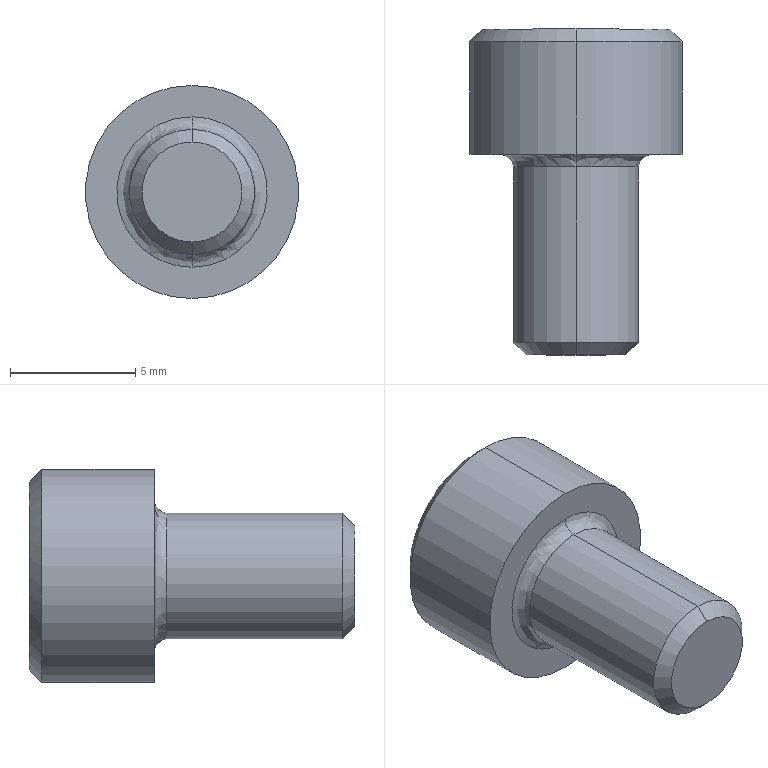Part | STEP file | 1 solid | 20 faces | box 8.5 x 13 x 8.5 mm | volume 400.62 mm3 | plane 10 | cone 4 | cylinder 4 | spline 2 | commonest cylinder face diameters 5 x2 8.5 x2
STEP:
#1=CARTESIAN_POINT('',(0.,0.,0.));
#2=DIRECTION('',(0.,0.,1.));
#3=DIRECTION('',(1.,0.,0.));
#4=AXIS2_PLACEMENT_3D('',#1,#2,#3);
#5=CARTESIAN_POINT('',(0.,-8.,2.));
#6=VERTEX_POINT('',#5);
#7=CARTESIAN_POINT('',(0.,-8.,-2.));
#8=VERTEX_POINT('',#7);
#9=CARTESIAN_POINT('',(0.,-8.,0.));
#10=DIRECTION('',(0.,1.,0.));
#11=DIRECTION('',(0.,0.,1.));
#12=AXIS2_PLACEMENT_3D('',#9,#10,#11);
#13=CIRCLE('',#12,2.);
#14=CARTESIAN_POINT('',(0.,-8.,0.));
#15=DIRECTION('',(0.,-1.,0.));
#16=DIRECTION('',(0.,0.,-1.));
#17=AXIS2_PLACEMENT_3D('',#14,#15,#16);
#18=PLANE('',#17);
#19=CARTESIAN_POINT('',(-2.,0.));
#20=CARTESIAN_POINT('',(-2.,3.464));
#21=CARTESIAN_POINT('',(1.,1.732));
#22=CARTESIAN_POINT('',(4.,0.));
#23=CARTESIAN_POINT('',(1.,-1.732));
#24=CARTESIAN_POINT('',(-2.,-3.464));
#25=CARTESIAN_POINT('',(-2.,0.));
#26=(BOUNDED_CURVE()B_SPLINE_CURVE(2,(#19,#20,#21,#22,#23,#24,#25),.UNSPECIFIED.,.T.,.F.)B_SPLINE_CURVE_WITH_KNOTS((1,2,2,2,2,1),(-2.094,0.,2.094,4.189,6.283,8.378),.UNSPECIFIED.)CURVE()GEOMETRIC_REPRESENTATION_ITEM()RATIONAL_B_SPLINE_CURVE((1.,0.5,1.,0.5,1.,0.5,1.))REPRESENTATION_ITEM(''));
#27=(GEOMETRIC_REPRESENTATION_CONTEXT(2)PARAMETRIC_REPRESENTATION_CONTEXT()REPRESENTATION_CONTEXT('',''));
#28=DEFINITIONAL_REPRESENTATION('',(#26),#27);
#29=PCURVE('',#18,#28);
#30=CARTESIAN_POINT('',(0.,-7.5,0.));
#31=DIRECTION('',(0.,1.,0.));
#32=DIRECTION('',(0.,0.,1.));
#33=AXIS2_PLACEMENT_3D('',#30,#31,#32);
#34=CONICAL_SURFACE('',#33,2.5,0.7854);
#35=CARTESIAN_POINT('',(0.,-0.5));
#36=DIRECTION('',(1.,0.));
#37=VECTOR('',#36,1.);
#38=LINE('',#35,#37);
#39=(GEOMETRIC_REPRESENTATION_CONTEXT(2)PARAMETRIC_REPRESENTATION_CONTEXT()REPRESENTATION_CONTEXT('',''));
#40=DEFINITIONAL_REPRESENTATION('',(#38),#39);
#41=PCURVE('',#34,#40);
#42=SURFACE_CURVE('',#13,(#29,#41),.PCURVE_S1.);
#43=EDGE_CURVE('',#6,#8,#42,.T.);
#44=ORIENTED_EDGE('',*,*,#43,.F.);
#45=CARTESIAN_POINT('',(0.,-8.,0.));
#46=DIRECTION('',(0.,1.,0.));
#47=DIRECTION('',(0.,0.,1.));
#48=AXIS2_PLACEMENT_3D('',#45,#46,#47);
#49=CIRCLE('',#48,2.);
#50=CARTESIAN_POINT('',(-2.,0.));
#51=CARTESIAN_POINT('',(-2.,3.464));
#52=CARTESIAN_POINT('',(1.,1.732));
#53=CARTESIAN_POINT('',(4.,0.));
#54=CARTESIAN_POINT('',(1.,-1.732));
#55=CARTESIAN_POINT('',(-2.,-3.464));
#56=CARTESIAN_POINT('',(-2.,0.));
#57=(BOUNDED_CURVE()B_SPLINE_CURVE(2,(#50,#51,#52,#53,#54,#55,#56),.UNSPECIFIED.,.T.,.F.)B_SPLINE_CURVE_WITH_KNOTS((1,2,2,2,2,1),(-2.094,0.,2.094,4.189,6.283,8.378),.UNSPECIFIED.)CURVE()GEOMETRIC_REPRESENTATION_ITEM()RATIONAL_B_SPLINE_CURVE((1.,0.5,1.,0.5,1.,0.5,1.))REPRESENTATION_ITEM(''));
#58=(GEOMETRIC_REPRESENTATION_CONTEXT(2)PARAMETRIC_REPRESENTATION_CONTEXT()REPRESENTATION_CONTEXT('',''));
#59=DEFINITIONAL_REPRESENTATION('',(#57),#58);
#60=PCURVE('',#18,#59);
#61=CARTESIAN_POINT('',(0.,-7.5,0.));
#62=DIRECTION('',(0.,1.,0.));
#63=DIRECTION('',(0.,0.,1.));
#64=AXIS2_PLACEMENT_3D('',#61,#62,#63);
#65=CONICAL_SURFACE('',#64,2.5,0.7854);
#66=CARTESIAN_POINT('',(0.,-0.5));
#67=DIRECTION('',(1.,0.));
#68=VECTOR('',#67,1.);
#69=LINE('',#66,#68);
#70=(GEOMETRIC_REPRESENTATION_CONTEXT(2)PARAMETRIC_REPRESENTATION_CONTEXT()REPRESENTATION_CONTEXT('',''));
#71=DEFINITIONAL_REPRESENTATION('',(#69),#70);
#72=PCURVE('',#65,#71);
#73=SURFACE_CURVE('',#49,(#60,#72),.PCURVE_S1.);
#74=EDGE_CURVE('',#8,#6,#73,.T.);
#75=ORIENTED_EDGE('',*,*,#74,.F.);
#76=EDGE_LOOP('',(#44,#75));
#77=FACE_BOUND('',#76,.T.);
#78=ADVANCED_FACE('',(#77),#18,.T.);
#79=CARTESIAN_POINT('',(-1.155,2.4,2.));
#80=VERTEX_POINT('',#79);
#81=CARTESIAN_POINT('',(1.155,2.4,2.));
#82=VERTEX_POINT('',#81);
#83=CARTESIAN_POINT('',(-1.155,2.4,2.));
#84=DIRECTION('',(1.,0.,0.));
#85=VECTOR('',#84,1.);
#86=LINE('',#83,#85);
#87=CARTESIAN_POINT('',(0.,2.4,0.));
#88=DIRECTION('',(0.,1.,0.));
#89=DIRECTION('',(1.,0.,0.));
#90=AXIS2_PLACEMENT_3D('',#87,#88,#89);
#91=PLANE('',#90);
#92=CARTESIAN_POINT('',(-1.155,-2.));
#93=DIRECTION('',(1.,0.));
#94=VECTOR('',#93,1.);
#95=LINE('',#92,#94);
#96=(GEOMETRIC_REPRESENTATION_CONTEXT(2)PARAMETRIC_REPRESENTATION_CONTEXT()REPRESENTATION_CONTEXT('',''));
#97=DEFINITIONAL_REPRESENTATION('',(#95),#96);
#98=PCURVE('',#91,#97);
#99=CARTESIAN_POINT('',(-1.155,2.4,2.));
#100=DIRECTION('',(0.,0.,1.));
#101=DIRECTION('',(1.,0.,0.));
#102=AXIS2_PLACEMENT_3D('',#99,#100,#101);
#103=PLANE('',#102);
#104=CARTESIAN_POINT('',(0.,0.));
#105=DIRECTION('',(1.,0.));
#106=VECTOR('',#105,1.);
#107=LINE('',#104,#106);
#108=(GEOMETRIC_REPRESENTATION_CONTEXT(2)PARAMETRIC_REPRESENTATION_CONTEXT()REPRESENTATION_CONTEXT('',''));
#109=DEFINITIONAL_REPRESENTATION('',(#107),#108);
#110=PCURVE('',#103,#109);
#111=SURFACE_CURVE('',#86,(#98,#110),.PCURVE_S1.);
#112=EDGE_CURVE('',#80,#82,#111,.T.);
#113=ORIENTED_EDGE('',*,*,#112,.T.);
#114=CARTESIAN_POINT('',(2.309,2.4,0.));
#115=VERTEX_POINT('',#114);
#116=CARTESIAN_POINT('',(1.155,2.4,2.));
#117=DIRECTION('',(0.5,0.,-0.866));
#118=VECTOR('',#117,1.);
#119=LINE('',#116,#118);
#120=CARTESIAN_POINT('',(1.155,-2.));
#121=DIRECTION('',(0.5,0.866));
#122=VECTOR('',#121,1.);
#123=LINE('',#120,#122);
#124=(GEOMETRIC_REPRESENTATION_CONTEXT(2)PARAMETRIC_REPRESENTATION_CONTEXT()REPRESENTATION_CONTEXT('',''));
#125=DEFINITIONAL_REPRESENTATION('',(#123),#124);
#126=PCURVE('',#91,#125);
#127=CARTESIAN_POINT('',(1.155,2.4,2.));
#128=DIRECTION('',(0.866,0.,0.5));
#129=DIRECTION('',(0.,-1.,0.));
#130=AXIS2_PLACEMENT_3D('',#127,#128,#129);
#131=PLANE('',#130);
#132=CARTESIAN_POINT('',(0.,0.));
#133=DIRECTION('',(0.,1.));
#134=VECTOR('',#133,1.);
#135=LINE('',#132,#134);
#136=(GEOMETRIC_REPRESENTATION_CONTEXT(2)PARAMETRIC_REPRESENTATION_CONTEXT()REPRESENTATION_CONTEXT('',''));
#137=DEFINITIONAL_REPRESENTATION('',(#135),#136);
#138=PCURVE('',#131,#137);
#139=SURFACE_CURVE('',#119,(#126,#138),.PCURVE_S1.);
#140=EDGE_CURVE('',#82,#115,#139,.T.);
#141=ORIENTED_EDGE('',*,*,#140,.T.);
#142=CARTESIAN_POINT('',(1.155,2.4,-2.));
#143=VERTEX_POINT('',#142);
#144=CARTESIAN_POINT('',(2.309,2.4,0.));
#145=DIRECTION('',(-0.5,0.,-0.866));
#146=VECTOR('',#145,1.);
#147=LINE('',#144,#146);
#148=CARTESIAN_POINT('',(2.309,0.));
#149=DIRECTION('',(-0.5,0.866));
#150=VECTOR('',#149,1.);
#151=LINE('',#148,#150);
#152=(GEOMETRIC_REPRESENTATION_CONTEXT(2)PARAMETRIC_REPRESENTATION_CONTEXT()REPRESENTATION_CONTEXT('',''));
#153=DEFINITIONAL_REPRESENTATION('',(#151),#152);
#154=PCURVE('',#91,#153);
#155=CARTESIAN_POINT('',(2.309,2.4,0.));
#156=DIRECTION('',(0.866,0.,-0.5));
#157=DIRECTION('',(0.,-1.,0.));
#158=AXIS2_PLACEMENT_3D('',#155,#156,#157);
#159=PLANE('',#158);
#160=CARTESIAN_POINT('',(0.,0.));
#161=DIRECTION('',(0.,1.));
#162=VECTOR('',#161,1.);
#163=LINE('',#160,#162);
#164=(GEOMETRIC_REPRESENTATION_CONTEXT(2)PARAMETRIC_REPRESENTATION_CONTEXT()REPRESENTATION_CONTEXT('',''));
#165=DEFINITIONAL_REPRESENTATION('',(#163),#164);
#166=PCURVE('',#159,#165);
#167=SURFACE_CURVE('',#147,(#154,#166),.PCURVE_S1.);
#168=EDGE_CURVE('',#115,#143,#167,.T.);
#169=ORIENTED_EDGE('',*,*,#168,.T.);
#170=CARTESIAN_POINT('',(-1.155,2.4,-2.));
#171=VERTEX_POINT('',#170);
#172=CARTESIAN_POINT('',(1.155,2.4,-2.));
#173=DIRECTION('',(-1.,0.,0.));
#174=VECTOR('',#173,1.);
#175=LINE('',#172,#174);
#176=CARTESIAN_POINT('',(1.155,2.));
#177=DIRECTION('',(-1.,0.));
#178=VECTOR('',#177,1.);
#179=LINE('',#176,#178);
#180=(GEOMETRIC_REPRESENTATION_CONTEXT(2)PARAMETRIC_REPRESENTATION_CONTEXT()REPRESENTATION_CONTEXT('',''));
#181=DEFINITIONAL_REPRESENTATION('',(#179),#180);
#182=PCURVE('',#91,#181);
#183=CARTESIAN_POINT('',(1.155,2.4,-2.));
#184=DIRECTION('',(0.,0.,-1.));
#185=DIRECTION('',(0.,-1.,0.));
#186=AXIS2_PLACEMENT_3D('',#183,#184,#185);
#187=PLANE('',#186);
#188=CARTESIAN_POINT('',(0.,0.));
#189=DIRECTION('',(0.,1.));
#190=VECTOR('',#189,1.);
#191=LINE('',#188,#190);
#192=(GEOMETRIC_REPRESENTATION_CONTEXT(2)PARAMETRIC_REPRESENTATION_CONTEXT()REPRESENTATION_CONTEXT('',''));
#193=DEFINITIONAL_REPRESENTATION('',(#191),#192);
#194=PCURVE('',#187,#193);
#195=SURFACE_CURVE('',#175,(#182,#194),.PCURVE_S1.);
#196=EDGE_CURVE('',#143,#171,#195,.T.);
#197=ORIENTED_EDGE('',*,*,#196,.T.);
#198=CARTESIAN_POINT('',(-2.309,2.4,0.));
#199=VERTEX_POINT('',#198);
#200=CARTESIAN_POINT('',(-1.155,2.4,-2.));
#201=DIRECTION('',(-0.5,0.,0.866));
#202=VECTOR('',#201,1.);
#203=LINE('',#200,#202);
#204=CARTESIAN_POINT('',(-1.155,2.));
#205=DIRECTION('',(-0.5,-0.866));
#206=VECTOR('',#205,1.);
#207=LINE('',#204,#206);
#208=(GEOMETRIC_REPRESENTATION_CONTEXT(2)PARAMETRIC_REPRESENTATION_CONTEXT()REPRESENTATION_CONTEXT('',''));
#209=DEFINITIONAL_REPRESENTATION('',(#207),#208);
#210=PCURVE('',#91,#209);
#211=CARTESIAN_POINT('',(-1.155,2.4,-2.));
#212=DIRECTION('',(-0.866,0.,-0.5));
#213=DIRECTION('',(-0.5,0.,0.866));
#214=AXIS2_PLACEMENT_3D('',#211,#212,#213);
#215=PLANE('',#214);
#216=CARTESIAN_POINT('',(0.,0.));
#217=DIRECTION('',(1.,0.));
#218=VECTOR('',#217,1.);
#219=LINE('',#216,#218);
#220=(GEOMETRIC_REPRESENTATION_CONTEXT(2)PARAMETRIC_REPRESENTATION_CONTEXT()REPRESENTATION_CONTEXT('',''));
#221=DEFINITIONAL_REPRESENTATION('',(#219),#220);
#222=PCURVE('',#215,#221);
#223=SURFACE_CURVE('',#203,(#210,#222),.PCURVE_S1.);
#224=EDGE_CURVE('',#171,#199,#223,.T.);
#225=ORIENTED_EDGE('',*,*,#224,.T.);
#226=CARTESIAN_POINT('',(-2.309,2.4,0.));
#227=DIRECTION('',(0.5,0.,0.866));
#228=VECTOR('',#227,1.);
#229=LINE('',#226,#228);
#230=CARTESIAN_POINT('',(-2.309,0.));
#231=DIRECTION('',(0.5,-0.866));
#232=VECTOR('',#231,1.);
#233=LINE('',#230,#232);
#234=(GEOMETRIC_REPRESENTATION_CONTEXT(2)PARAMETRIC_REPRESENTATION_CONTEXT()REPRESENTATION_CONTEXT('',''));
#235=DEFINITIONAL_REPRESENTATION('',(#233),#234);
#236=PCURVE('',#91,#235);
#237=CARTESIAN_POINT('',(-2.309,2.4,0.));
#238=DIRECTION('',(-0.866,0.,0.5));
#239=DIRECTION('',(0.,1.,0.));
#240=AXIS2_PLACEMENT_3D('',#237,#238,#239);
#241=PLANE('',#240);
#242=CARTESIAN_POINT('',(0.,0.));
#243=DIRECTION('',(0.,-1.));
#244=VECTOR('',#243,1.);
#245=LINE('',#242,#244);
#246=(GEOMETRIC_REPRESENTATION_CONTEXT(2)PARAMETRIC_REPRESENTATION_CONTEXT()REPRESENTATION_CONTEXT('',''));
#247=DEFINITIONAL_REPRESENTATION('',(#245),#246);
#248=PCURVE('',#241,#247);
#249=SURFACE_CURVE('',#229,(#236,#248),.PCURVE_S1.);
#250=EDGE_CURVE('',#199,#80,#249,.T.);
#251=ORIENTED_EDGE('',*,*,#250,.T.);
#252=EDGE_LOOP('',(#113,#141,#169,#197,#225,#251));
#253=FACE_BOUND('',#252,.T.);
#254=ADVANCED_FACE('',(#253),#91,.T.);
#255=CARTESIAN_POINT('',(0.,-7.5,-2.5));
#256=VERTEX_POINT('',#255);
#257=CARTESIAN_POINT('',(0.,-7.5,-2.5));
#258=DIRECTION('',(0.,0.7071,-0.7071));
#259=VECTOR('',#258,1.);
#260=LINE('',#257,#259);
#261=CARTESIAN_POINT('',(3.142,0.));
#262=DIRECTION('',(0.,1.));
#263=VECTOR('',#262,1.);
#264=LINE('',#261,#263);
#265=(GEOMETRIC_REPRESENTATION_CONTEXT(2)PARAMETRIC_REPRESENTATION_CONTEXT()REPRESENTATION_CONTEXT('',''));
#266=DEFINITIONAL_REPRESENTATION('',(#264),#265);
#267=PCURVE('',#65,#266);
#268=CARTESIAN_POINT('',(3.142,0.));
#269=DIRECTION('',(0.,1.));
#270=VECTOR('',#269,1.);
#271=LINE('',#268,#270);
#272=(GEOMETRIC_REPRESENTATION_CONTEXT(2)PARAMETRIC_REPRESENTATION_CONTEXT()REPRESENTATION_CONTEXT('',''));
#273=DEFINITIONAL_REPRESENTATION('',(#271),#272);
#274=PCURVE('',#34,#273);
#275=SURFACE_CURVE('',#260,(#267,#274),.PCURVE_S1.);
#276=EDGE_CURVE('',#8,#256,#275,.T.);
#277=ORIENTED_EDGE('',*,*,#276,.F.);
#278=ORIENTED_EDGE('',*,*,#74,.T.);
#279=CARTESIAN_POINT('',(0.,-7.5,2.5));
#280=VERTEX_POINT('',#279);
#281=CARTESIAN_POINT('',(0.,-7.5,2.5));
#282=DIRECTION('',(0.,0.7071,0.7071));
#283=VECTOR('',#282,1.);
#284=LINE('',#281,#283);
#285=CARTESIAN_POINT('',(6.283,0.));
#286=DIRECTION('',(0.,1.));
#287=VECTOR('',#286,1.);
#288=LINE('',#285,#287);
#289=(GEOMETRIC_REPRESENTATION_CONTEXT(2)PARAMETRIC_REPRESENTATION_CONTEXT()REPRESENTATION_CONTEXT('',''));
#290=DEFINITIONAL_REPRESENTATION('',(#288),#289);
#291=PCURVE('',#65,#290);
#292=CARTESIAN_POINT('',(0.,0.));
#293=DIRECTION('',(0.,1.));
#294=VECTOR('',#293,1.);
#295=LINE('',#292,#294);
#296=(GEOMETRIC_REPRESENTATION_CONTEXT(2)PARAMETRIC_REPRESENTATION_CONTEXT()REPRESENTATION_CONTEXT('',''));
#297=DEFINITIONAL_REPRESENTATION('',(#295),#296);
#298=PCURVE('',#34,#297);
#299=SURFACE_CURVE('',#284,(#291,#298),.PCURVE_S1.);
#300=EDGE_CURVE('',#6,#280,#299,.T.);
#301=ORIENTED_EDGE('',*,*,#300,.T.);
#302=CARTESIAN_POINT('',(0.,-7.5,0.));
#303=DIRECTION('',(0.,1.,0.));
#304=DIRECTION('',(0.,0.,1.));
#305=AXIS2_PLACEMENT_3D('',#302,#303,#304);
#306=CIRCLE('',#305,2.5);
#307=CARTESIAN_POINT('',(0.,0.));
#308=DIRECTION('',(1.,0.));
#309=VECTOR('',#308,1.);
#310=LINE('',#307,#309);
#311=(GEOMETRIC_REPRESENTATION_CONTEXT(2)PARAMETRIC_REPRESENTATION_CONTEXT()REPRESENTATION_CONTEXT('',''));
#312=DEFINITIONAL_REPRESENTATION('',(#310),#311);
#313=PCURVE('',#65,#312);
#314=CARTESIAN_POINT('',(0.,-8.,0.));
#315=DIRECTION('',(0.,1.,0.));
#316=DIRECTION('',(0.,0.,1.));
#317=AXIS2_PLACEMENT_3D('',#314,#315,#316);
#318=CYLINDRICAL_SURFACE('',#317,2.5);
#319=CARTESIAN_POINT('',(0.,0.5));
#320=DIRECTION('',(1.,0.));
#321=VECTOR('',#320,1.);
#322=LINE('',#319,#321);
#323=(GEOMETRIC_REPRESENTATION_CONTEXT(2)PARAMETRIC_REPRESENTATION_CONTEXT()REPRESENTATION_CONTEXT('',''));
#324=DEFINITIONAL_REPRESENTATION('',(#322),#323);
#325=PCURVE('',#318,#324);
#326=SURFACE_CURVE('',#306,(#313,#325),.PCURVE_S1.);
#327=EDGE_CURVE('',#256,#280,#326,.T.);
#328=ORIENTED_EDGE('',*,*,#327,.F.);
#329=EDGE_LOOP('',(#277,#278,#301,#328));
#330=FACE_BOUND('',#329,.T.);
#331=ADVANCED_FACE('',(#330),#65,.T.);
#332=CARTESIAN_POINT('',(1.155,5.,-2.));
#333=VERTEX_POINT('',#332);
#334=CARTESIAN_POINT('',(1.155,2.4,-2.));
#335=DIRECTION('',(0.,-1.,0.));
#336=VECTOR('',#335,1.);
#337=LINE('',#334,#336);
#338=CARTESIAN_POINT('',(0.,2.309));
#339=DIRECTION('',(1.,0.));
#340=VECTOR('',#339,1.);
#341=LINE('',#338,#340);
#342=(GEOMETRIC_REPRESENTATION_CONTEXT(2)PARAMETRIC_REPRESENTATION_CONTEXT()REPRESENTATION_CONTEXT('',''));
#343=DEFINITIONAL_REPRESENTATION('',(#341),#342);
#344=PCURVE('',#159,#343);
#345=CARTESIAN_POINT('',(0.,0.));
#346=DIRECTION('',(1.,0.));
#347=VECTOR('',#346,1.);
#348=LINE('',#345,#347);
#349=(GEOMETRIC_REPRESENTATION_CONTEXT(2)PARAMETRIC_REPRESENTATION_CONTEXT()REPRESENTATION_CONTEXT('',''));
#350=DEFINITIONAL_REPRESENTATION('',(#348),#349);
#351=PCURVE('',#187,#350);
#352=SURFACE_CURVE('',#337,(#344,#351),.PCURVE_S1.);
#353=EDGE_CURVE('',#333,#143,#352,.T.);
#354=ORIENTED_EDGE('',*,*,#353,.T.);
#355=ORIENTED_EDGE('',*,*,#168,.F.);
#356=CARTESIAN_POINT('',(2.309,5.,0.));
#357=VERTEX_POINT('',#356);
#358=CARTESIAN_POINT('',(2.309,2.4,0.));
#359=DIRECTION('',(0.,1.,0.));
#360=VECTOR('',#359,1.);
#361=LINE('',#358,#360);
#362=CARTESIAN_POINT('',(0.,0.));
#363=DIRECTION('',(-1.,0.));
#364=VECTOR('',#363,1.);
#365=LINE('',#362,#364);
#366=(GEOMETRIC_REPRESENTATION_CONTEXT(2)PARAMETRIC_REPRESENTATION_CONTEXT()REPRESENTATION_CONTEXT('',''));
#367=DEFINITIONAL_REPRESENTATION('',(#365),#366);
#368=PCURVE('',#159,#367);
#369=CARTESIAN_POINT('',(0.,2.309));
#370=DIRECTION('',(-1.,0.));
#371=VECTOR('',#370,1.);
#372=LINE('',#369,#371);
#373=(GEOMETRIC_REPRESENTATION_CONTEXT(2)PARAMETRIC_REPRESENTATION_CONTEXT()REPRESENTATION_CONTEXT('',''));
#374=DEFINITIONAL_REPRESENTATION('',(#372),#373);
#375=PCURVE('',#131,#374);
#376=SURFACE_CURVE('',#361,(#368,#375),.PCURVE_S1.);
#377=EDGE_CURVE('',#115,#357,#376,.T.);
#378=ORIENTED_EDGE('',*,*,#377,.T.);
#379=CARTESIAN_POINT('',(1.155,5.,-2.));
#380=DIRECTION('',(0.5,0.,0.866));
#381=VECTOR('',#380,1.);
#382=LINE('',#379,#381);
#383=CARTESIAN_POINT('',(-2.6,2.309));
#384=DIRECTION('',(0.,-1.));
#385=VECTOR('',#384,1.);
#386=LINE('',#383,#385);
#387=(GEOMETRIC_REPRESENTATION_CONTEXT(2)PARAMETRIC_REPRESENTATION_CONTEXT()REPRESENTATION_CONTEXT('',''));
#388=DEFINITIONAL_REPRESENTATION('',(#386),#387);
#389=PCURVE('',#159,#388);
#390=CARTESIAN_POINT('',(0.,5.,0.));
#391=DIRECTION('',(0.,1.,0.));
#392=DIRECTION('',(1.,0.,0.));
#393=AXIS2_PLACEMENT_3D('',#390,#391,#392);
#394=PLANE('',#393);
#395=CARTESIAN_POINT('',(1.155,2.));
#396=DIRECTION('',(0.5,-0.866));
#397=VECTOR('',#396,1.);
#398=LINE('',#395,#397);
#399=(GEOMETRIC_REPRESENTATION_CONTEXT(2)PARAMETRIC_REPRESENTATION_CONTEXT()REPRESENTATION_CONTEXT('',''));
#400=DEFINITIONAL_REPRESENTATION('',(#398),#399);
#401=PCURVE('',#394,#400);
#402=SURFACE_CURVE('',#382,(#389,#401),.PCURVE_S1.);
#403=EDGE_CURVE('',#333,#357,#402,.T.);
#404=ORIENTED_EDGE('',*,*,#403,.F.);
#405=EDGE_LOOP('',(#354,#355,#378,#404));
#406=FACE_BOUND('',#405,.T.);
#407=ADVANCED_FACE('',(#406),#159,.F.);
#408=ORIENTED_EDGE('',*,*,#377,.F.);
#409=ORIENTED_EDGE('',*,*,#140,.F.);
#410=CARTESIAN_POINT('',(1.155,5.,2.));
#411=VERTEX_POINT('',#410);
#412=CARTESIAN_POINT('',(1.155,2.4,2.));
#413=DIRECTION('',(0.,1.,0.));
#414=VECTOR('',#413,1.);
#415=LINE('',#412,#414);
#416=CARTESIAN_POINT('',(0.,0.));
#417=DIRECTION('',(-1.,0.));
#418=VECTOR('',#417,1.);
#419=LINE('',#416,#418);
#420=(GEOMETRIC_REPRESENTATION_CONTEXT(2)PARAMETRIC_REPRESENTATION_CONTEXT()REPRESENTATION_CONTEXT('',''));
#421=DEFINITIONAL_REPRESENTATION('',(#419),#420);
#422=PCURVE('',#131,#421);
#423=CARTESIAN_POINT('',(2.309,0.));
#424=DIRECTION('',(0.,1.));
#425=VECTOR('',#424,1.);
#426=LINE('',#423,#425);
#427=(GEOMETRIC_REPRESENTATION_CONTEXT(2)PARAMETRIC_REPRESENTATION_CONTEXT()REPRESENTATION_CONTEXT('',''));
#428=DEFINITIONAL_REPRESENTATION('',(#426),#427);
#429=PCURVE('',#103,#428);
#430=SURFACE_CURVE('',#415,(#422,#429),.PCURVE_S1.);
#431=EDGE_CURVE('',#82,#411,#430,.T.);
#432=ORIENTED_EDGE('',*,*,#431,.T.);
#433=CARTESIAN_POINT('',(2.309,5.,0.));
#434=DIRECTION('',(-0.5,0.,0.866));
#435=VECTOR('',#434,1.);
#436=LINE('',#433,#435);
#437=CARTESIAN_POINT('',(-2.6,2.309));
#438=DIRECTION('',(0.,-1.));
#439=VECTOR('',#438,1.);
#440=LINE('',#437,#439);
#441=(GEOMETRIC_REPRESENTATION_CONTEXT(2)PARAMETRIC_REPRESENTATION_CONTEXT()REPRESENTATION_CONTEXT('',''));
#442=DEFINITIONAL_REPRESENTATION('',(#440),#441);
#443=PCURVE('',#131,#442);
#444=CARTESIAN_POINT('',(2.309,0.));
#445=DIRECTION('',(-0.5,-0.866));
#446=VECTOR('',#445,1.);
#447=LINE('',#444,#446);
#448=(GEOMETRIC_REPRESENTATION_CONTEXT(2)PARAMETRIC_REPRESENTATION_CONTEXT()REPRESENTATION_CONTEXT('',''));
#449=DEFINITIONAL_REPRESENTATION('',(#447),#448);
#450=PCURVE('',#394,#449);
#451=SURFACE_CURVE('',#436,(#443,#450),.PCURVE_S1.);
#452=EDGE_CURVE('',#357,#411,#451,.T.);
#453=ORIENTED_EDGE('',*,*,#452,.F.);
#454=EDGE_LOOP('',(#408,#409,#432,#453));
#455=FACE_BOUND('',#454,.T.);
#456=ADVANCED_FACE('',(#455),#131,.F.);
#457=ORIENTED_EDGE('',*,*,#431,.F.);
#458=ORIENTED_EDGE('',*,*,#112,.F.);
#459=CARTESIAN_POINT('',(-1.155,5.,2.));
#460=VERTEX_POINT('',#459);
#461=CARTESIAN_POINT('',(-1.155,2.4,2.));
#462=DIRECTION('',(0.,1.,0.));
#463=VECTOR('',#462,1.);
#464=LINE('',#461,#463);
#465=CARTESIAN_POINT('',(0.,0.));
#466=DIRECTION('',(0.,1.));
#467=VECTOR('',#466,1.);
#468=LINE('',#465,#467);
#469=(GEOMETRIC_REPRESENTATION_CONTEXT(2)PARAMETRIC_REPRESENTATION_CONTEXT()REPRESENTATION_CONTEXT('',''));
#470=DEFINITIONAL_REPRESENTATION('',(#468),#469);
#471=PCURVE('',#103,#470);
#472=CARTESIAN_POINT('',(0.,-2.309));
#473=DIRECTION('',(1.,0.));
#474=VECTOR('',#473,1.);
#475=LINE('',#472,#474);
#476=(GEOMETRIC_REPRESENTATION_CONTEXT(2)PARAMETRIC_REPRESENTATION_CONTEXT()REPRESENTATION_CONTEXT('',''));
#477=DEFINITIONAL_REPRESENTATION('',(#475),#476);
#478=PCURVE('',#241,#477);
#479=SURFACE_CURVE('',#464,(#471,#478),.PCURVE_S1.);
#480=EDGE_CURVE('',#80,#460,#479,.T.);
#481=ORIENTED_EDGE('',*,*,#480,.T.);
#482=CARTESIAN_POINT('',(0.,5.,2.));
#483=DIRECTION('',(-1.,0.,0.));
#484=VECTOR('',#483,1.);
#485=LINE('',#482,#484);
#486=CARTESIAN_POINT('',(1.155,2.6));
#487=DIRECTION('',(-1.,0.));
#488=VECTOR('',#487,1.);
#489=LINE('',#486,#488);
#490=(GEOMETRIC_REPRESENTATION_CONTEXT(2)PARAMETRIC_REPRESENTATION_CONTEXT()REPRESENTATION_CONTEXT('',''));
#491=DEFINITIONAL_REPRESENTATION('',(#489),#490);
#492=PCURVE('',#103,#491);
#493=CARTESIAN_POINT('',(0.,-2.));
#494=DIRECTION('',(-1.,0.));
#495=VECTOR('',#494,1.);
#496=LINE('',#493,#495);
#497=(GEOMETRIC_REPRESENTATION_CONTEXT(2)PARAMETRIC_REPRESENTATION_CONTEXT()REPRESENTATION_CONTEXT('',''));
#498=DEFINITIONAL_REPRESENTATION('',(#496),#497);
#499=PCURVE('',#394,#498);
#500=SURFACE_CURVE('',#485,(#492,#499),.PCURVE_S1.);
#501=EDGE_CURVE('',#411,#460,#500,.T.);
#502=ORIENTED_EDGE('',*,*,#501,.F.);
#503=EDGE_LOOP('',(#457,#458,#481,#502));
#504=FACE_BOUND('',#503,.T.);
#505=ADVANCED_FACE('',(#504),#103,.F.);
#506=ORIENTED_EDGE('',*,*,#480,.F.);
#507=ORIENTED_EDGE('',*,*,#250,.F.);
#508=CARTESIAN_POINT('',(-2.309,5.,0.));
#509=VERTEX_POINT('',#508);
#510=CARTESIAN_POINT('',(-2.309,2.4,0.));
#511=DIRECTION('',(0.,1.,0.));
#512=VECTOR('',#511,1.);
#513=LINE('',#510,#512);
#514=CARTESIAN_POINT('',(0.,0.));
#515=DIRECTION('',(1.,0.));
#516=VECTOR('',#515,1.);
#517=LINE('',#514,#516);
#518=(GEOMETRIC_REPRESENTATION_CONTEXT(2)PARAMETRIC_REPRESENTATION_CONTEXT()REPRESENTATION_CONTEXT('',''));
#519=DEFINITIONAL_REPRESENTATION('',(#517),#518);
#520=PCURVE('',#241,#519);
#521=CARTESIAN_POINT('',(2.309,0.));
#522=DIRECTION('',(0.,1.));
#523=VECTOR('',#522,1.);
#524=LINE('',#521,#523);
#525=(GEOMETRIC_REPRESENTATION_CONTEXT(2)PARAMETRIC_REPRESENTATION_CONTEXT()REPRESENTATION_CONTEXT('',''));
#526=DEFINITIONAL_REPRESENTATION('',(#524),#525);
#527=PCURVE('',#215,#526);
#528=SURFACE_CURVE('',#513,(#520,#527),.PCURVE_S1.);
#529=EDGE_CURVE('',#199,#509,#528,.T.);
#530=ORIENTED_EDGE('',*,*,#529,.T.);
#531=CARTESIAN_POINT('',(-1.155,5.,2.));
#532=DIRECTION('',(-0.5,0.,-0.866));
#533=VECTOR('',#532,1.);
#534=LINE('',#531,#533);
#535=CARTESIAN_POINT('',(2.6,-2.309));
#536=DIRECTION('',(0.,1.));
#537=VECTOR('',#536,1.);
#538=LINE('',#535,#537);
#539=(GEOMETRIC_REPRESENTATION_CONTEXT(2)PARAMETRIC_REPRESENTATION_CONTEXT()REPRESENTATION_CONTEXT('',''));
#540=DEFINITIONAL_REPRESENTATION('',(#538),#539);
#541=PCURVE('',#241,#540);
#542=CARTESIAN_POINT('',(-1.155,-2.));
#543=DIRECTION('',(-0.5,0.866));
#544=VECTOR('',#543,1.);
#545=LINE('',#542,#544);
#546=(GEOMETRIC_REPRESENTATION_CONTEXT(2)PARAMETRIC_REPRESENTATION_CONTEXT()REPRESENTATION_CONTEXT('',''));
#547=DEFINITIONAL_REPRESENTATION('',(#545),#546);
#548=PCURVE('',#394,#547);
#549=SURFACE_CURVE('',#534,(#541,#548),.PCURVE_S1.);
#550=EDGE_CURVE('',#460,#509,#549,.T.);
#551=ORIENTED_EDGE('',*,*,#550,.F.);
#552=EDGE_LOOP('',(#506,#507,#530,#551));
#553=FACE_BOUND('',#552,.T.);
#554=ADVANCED_FACE('',(#553),#241,.F.);
#555=ORIENTED_EDGE('',*,*,#529,.F.);
#556=ORIENTED_EDGE('',*,*,#224,.F.);
#557=CARTESIAN_POINT('',(-1.155,5.,-2.));
#558=VERTEX_POINT('',#557);
#559=CARTESIAN_POINT('',(-1.155,2.4,-2.));
#560=DIRECTION('',(0.,1.,0.));
#561=VECTOR('',#560,1.);
#562=LINE('',#559,#561);
#563=CARTESIAN_POINT('',(0.,0.));
#564=DIRECTION('',(0.,1.));
#565=VECTOR('',#564,1.);
#566=LINE('',#563,#565);
#567=(GEOMETRIC_REPRESENTATION_CONTEXT(2)PARAMETRIC_REPRESENTATION_CONTEXT()REPRESENTATION_CONTEXT('',''));
#568=DEFINITIONAL_REPRESENTATION('',(#566),#567);
#569=PCURVE('',#215,#568);
#570=CARTESIAN_POINT('',(0.,2.309));
#571=DIRECTION('',(-1.,0.));
#572=VECTOR('',#571,1.);
#573=LINE('',#570,#572);
#574=(GEOMETRIC_REPRESENTATION_CONTEXT(2)PARAMETRIC_REPRESENTATION_CONTEXT()REPRESENTATION_CONTEXT('',''));
#575=DEFINITIONAL_REPRESENTATION('',(#573),#574);
#576=PCURVE('',#187,#575);
#577=SURFACE_CURVE('',#562,(#569,#576),.PCURVE_S1.);
#578=EDGE_CURVE('',#171,#558,#577,.T.);
#579=ORIENTED_EDGE('',*,*,#578,.T.);
#580=CARTESIAN_POINT('',(-2.309,5.,0.));
#581=DIRECTION('',(0.5,0.,-0.866));
#582=VECTOR('',#581,1.);
#583=LINE('',#580,#582);
#584=CARTESIAN_POINT('',(2.309,2.6));
#585=DIRECTION('',(-1.,0.));
#586=VECTOR('',#585,1.);
#587=LINE('',#584,#586);
#588=(GEOMETRIC_REPRESENTATION_CONTEXT(2)PARAMETRIC_REPRESENTATION_CONTEXT()REPRESENTATION_CONTEXT('',''));
#589=DEFINITIONAL_REPRESENTATION('',(#587),#588);
#590=PCURVE('',#215,#589);
#591=CARTESIAN_POINT('',(-2.309,0.));
#592=DIRECTION('',(0.5,0.866));
#593=VECTOR('',#592,1.);
#594=LINE('',#591,#593);
#595=(GEOMETRIC_REPRESENTATION_CONTEXT(2)PARAMETRIC_REPRESENTATION_CONTEXT()REPRESENTATION_CONTEXT('',''));
#596=DEFINITIONAL_REPRESENTATION('',(#594),#595);
#597=PCURVE('',#394,#596);
#598=SURFACE_CURVE('',#583,(#590,#597),.PCURVE_S1.);
#599=EDGE_CURVE('',#509,#558,#598,.T.);
#600=ORIENTED_EDGE('',*,*,#599,.F.);
#601=EDGE_LOOP('',(#555,#556,#579,#600));
#602=FACE_BOUND('',#601,.T.);
#603=ADVANCED_FACE('',(#602),#215,.F.);
#604=ORIENTED_EDGE('',*,*,#578,.F.);
#605=ORIENTED_EDGE('',*,*,#196,.F.);
#606=ORIENTED_EDGE('',*,*,#353,.F.);
#607=CARTESIAN_POINT('',(0.,5.,-2.));
#608=DIRECTION('',(1.,0.,0.));
#609=VECTOR('',#608,1.);
#610=LINE('',#607,#609);
#611=CARTESIAN_POINT('',(-2.6,1.155));
#612=DIRECTION('',(0.,-1.));
#613=VECTOR('',#612,1.);
#614=LINE('',#611,#613);
#615=(GEOMETRIC_REPRESENTATION_CONTEXT(2)PARAMETRIC_REPRESENTATION_CONTEXT()REPRESENTATION_CONTEXT('',''));
#616=DEFINITIONAL_REPRESENTATION('',(#614),#615);
#617=PCURVE('',#187,#616);
#618=CARTESIAN_POINT('',(0.,2.));
#619=DIRECTION('',(1.,0.));
#620=VECTOR('',#619,1.);
#621=LINE('',#618,#620);
#622=(GEOMETRIC_REPRESENTATION_CONTEXT(2)PARAMETRIC_REPRESENTATION_CONTEXT()REPRESENTATION_CONTEXT('',''));
#623=DEFINITIONAL_REPRESENTATION('',(#621),#622);
#624=PCURVE('',#394,#623);
#625=SURFACE_CURVE('',#610,(#617,#624),.PCURVE_S1.);
#626=EDGE_CURVE('',#558,#333,#625,.T.);
#627=ORIENTED_EDGE('',*,*,#626,.F.);
#628=EDGE_LOOP('',(#604,#605,#606,#627));
#629=FACE_BOUND('',#628,.T.);
#630=ADVANCED_FACE('',(#629),#187,.F.);
#631=CARTESIAN_POINT('',(0.,-0.5,-2.5));
#632=VERTEX_POINT('',#631);
#633=CARTESIAN_POINT('',(0.,-8.,-2.5));
#634=DIRECTION('',(0.,1.,0.));
#635=VECTOR('',#634,1.);
#636=LINE('',#633,#635);
#637=CARTESIAN_POINT('',(3.142,0.));
#638=DIRECTION('',(0.,1.));
#639=VECTOR('',#638,1.);
#640=LINE('',#637,#639);
#641=(GEOMETRIC_REPRESENTATION_CONTEXT(2)PARAMETRIC_REPRESENTATION_CONTEXT()REPRESENTATION_CONTEXT('',''));
#642=DEFINITIONAL_REPRESENTATION('',(#640),#641);
#643=PCURVE('',#318,#642);
#644=CARTESIAN_POINT('',(0.,-8.,0.));
#645=DIRECTION('',(0.,1.,0.));
#646=DIRECTION('',(0.,0.,1.));
#647=AXIS2_PLACEMENT_3D('',#644,#645,#646);
#648=CYLINDRICAL_SURFACE('',#647,2.5);
#649=CARTESIAN_POINT('',(3.142,0.));
#650=DIRECTION('',(0.,1.));
#651=VECTOR('',#650,1.);
#652=LINE('',#649,#651);
#653=(GEOMETRIC_REPRESENTATION_CONTEXT(2)PARAMETRIC_REPRESENTATION_CONTEXT()REPRESENTATION_CONTEXT('',''));
#654=DEFINITIONAL_REPRESENTATION('',(#652),#653);
#655=PCURVE('',#648,#654);
#656=SURFACE_CURVE('',#636,(#643,#655),.PCURVE_S1.);
#657=EDGE_CURVE('',#256,#632,#656,.T.);
#658=ORIENTED_EDGE('',*,*,#657,.F.);
#659=ORIENTED_EDGE('',*,*,#327,.T.);
#660=CARTESIAN_POINT('',(0.,-0.5,2.5));
#661=VERTEX_POINT('',#660);
#662=CARTESIAN_POINT('',(0.,-8.,2.5));
#663=DIRECTION('',(0.,1.,0.));
#664=VECTOR('',#663,1.);
#665=LINE('',#662,#664);
#666=CARTESIAN_POINT('',(6.283,0.));
#667=DIRECTION('',(0.,1.));
#668=VECTOR('',#667,1.);
#669=LINE('',#666,#668);
#670=(GEOMETRIC_REPRESENTATION_CONTEXT(2)PARAMETRIC_REPRESENTATION_CONTEXT()REPRESENTATION_CONTEXT('',''));
#671=DEFINITIONAL_REPRESENTATION('',(#669),#670);
#672=PCURVE('',#318,#671);
#673=CARTESIAN_POINT('',(0.,0.));
#674=DIRECTION('',(0.,1.));
#675=VECTOR('',#674,1.);
#676=LINE('',#673,#675);
#677=(GEOMETRIC_REPRESENTATION_CONTEXT(2)PARAMETRIC_REPRESENTATION_CONTEXT()REPRESENTATION_CONTEXT('',''));
#678=DEFINITIONAL_REPRESENTATION('',(#676),#677);
#679=PCURVE('',#648,#678);
#680=SURFACE_CURVE('',#665,(#672,#679),.PCURVE_S1.);
#681=EDGE_CURVE('',#280,#661,#680,.T.);
#682=ORIENTED_EDGE('',*,*,#681,.T.);
#683=CARTESIAN_POINT('',(0.,-0.5,0.));
#684=DIRECTION('',(0.,-1.,0.));
#685=DIRECTION('',(0.,0.,1.));
#686=AXIS2_PLACEMENT_3D('',#683,#684,#685);
#687=CIRCLE('',#686,2.5);
#688=CARTESIAN_POINT('',(6.283,7.5));
#689=DIRECTION('',(-1.,0.));
#690=VECTOR('',#689,1.);
#691=LINE('',#688,#690);
#692=(GEOMETRIC_REPRESENTATION_CONTEXT(2)PARAMETRIC_REPRESENTATION_CONTEXT()REPRESENTATION_CONTEXT('',''));
#693=DEFINITIONAL_REPRESENTATION('',(#691),#692);
#694=PCURVE('',#318,#693);
#695=CARTESIAN_POINT('',(0.,-0.5,-2.5));
#696=CARTESIAN_POINT('',(-5.,-0.5,-2.5));
#697=CARTESIAN_POINT('',(-5.,-0.5,2.5));
#698=CARTESIAN_POINT('',(0.,-0.5,2.5));
#699=CARTESIAN_POINT('',(0.,-0.2071,-2.5));
#700=CARTESIAN_POINT('',(-5.,-0.2071,-2.5));
#701=CARTESIAN_POINT('',(-5.,-0.2071,2.5));
#702=CARTESIAN_POINT('',(0.,-0.2071,2.5));
#703=CARTESIAN_POINT('',(0.,0.,-2.707));
#704=CARTESIAN_POINT('',(-5.414,0.,-2.707));
#705=CARTESIAN_POINT('',(-5.414,0.,2.707));
#706=CARTESIAN_POINT('',(0.,0.,2.707));
#707=CARTESIAN_POINT('',(0.,0.,-3.));
#708=CARTESIAN_POINT('',(-6.,0.,-3.));
#709=CARTESIAN_POINT('',(-6.,0.,3.));
#710=CARTESIAN_POINT('',(0.,0.,3.));
#711=(BOUNDED_SURFACE()B_SPLINE_SURFACE(3,3,((#695,#696,#697,#698),(#699,#700,#701,#702),(#703,#704,#705,#706),(#707,#708,#709,#710)),.UNSPECIFIED.,.F.,.F.,.F.)B_SPLINE_SURFACE_WITH_KNOTS((4,4),(4,4),(0.,1.),(0.,1.),.PIECEWISE_BEZIER_KNOTS.)GEOMETRIC_REPRESENTATION_ITEM()RATIONAL_B_SPLINE_SURFACE(((1.,0.3333,0.3333,1.),(0.8047,0.2682,0.2682,0.8047),(0.8047,0.2682,0.2682,0.8047),(1.,0.3333,0.3333,1.)))REPRESENTATION_ITEM('')SURFACE());
#712=CARTESIAN_POINT('',(0.,1.));
#713=CARTESIAN_POINT('',(0.,0.9763));
#714=CARTESIAN_POINT('',(0.,0.9319));
#715=CARTESIAN_POINT('',(0.,0.8733));
#716=CARTESIAN_POINT('',(0.,0.8206));
#717=CARTESIAN_POINT('',(0.,0.7724));
#718=CARTESIAN_POINT('',(0.,0.7279));
#719=CARTESIAN_POINT('',(0.,0.6861));
#720=CARTESIAN_POINT('',(0.,0.6465));
#721=CARTESIAN_POINT('',(0.,0.6086));
#722=CARTESIAN_POINT('',(0.,0.5718));
#723=CARTESIAN_POINT('',(0.,0.5357));
#724=CARTESIAN_POINT('',(0.,0.5));
#725=CARTESIAN_POINT('',(0.,0.4643));
#726=CARTESIAN_POINT('',(0.,0.4282));
#727=CARTESIAN_POINT('',(0.,0.3914));
#728=CARTESIAN_POINT('',(0.,0.3535));
#729=CARTESIAN_POINT('',(0.,0.3139));
#730=CARTESIAN_POINT('',(0.,0.2721));
#731=CARTESIAN_POINT('',(0.,0.2276));
#732=CARTESIAN_POINT('',(0.,0.1794));
#733=CARTESIAN_POINT('',(0.,0.1267));
#734=CARTESIAN_POINT('',(0.,0.06805));
#735=CARTESIAN_POINT('',(0.,0.02375));
#736=CARTESIAN_POINT('',(0.,0.));
#737=B_SPLINE_CURVE_WITH_KNOTS('',3,(#712,#713,#714,#715,#716,#717,#718,#719,#720,#721,#722,#723,#724,#725,#726,#727,#728,#729,#730,#731,#732,#733,#734,#735,#736),.UNSPECIFIED.,.F.,.F.,(4,1,1,1,1,1,1,1,1,1,1,1,1,1,1,1,1,1,1,1,1,1,4),(0.,0.1428,0.2856,0.4284,0.5712,0.714,0.8568,0.9996,1.142,1.285,1.428,1.571,1.714,1.856,1.999,2.142,2.285,2.428,2.57,2.713,2.856,2.999,3.142),.QUASI_UNIFORM_KNOTS.);
#738=(GEOMETRIC_REPRESENTATION_CONTEXT(2)PARAMETRIC_REPRESENTATION_CONTEXT()REPRESENTATION_CONTEXT('',''));
#739=DEFINITIONAL_REPRESENTATION('',(#737),#738);
#740=PCURVE('',#711,#739);
#741=SURFACE_CURVE('',#687,(#694,#740),.PCURVE_S1.);
#742=EDGE_CURVE('',#661,#632,#741,.T.);
#743=ORIENTED_EDGE('',*,*,#742,.T.);
#744=EDGE_LOOP('',(#658,#659,#682,#743));
#745=FACE_BOUND('',#744,.T.);
#746=ADVANCED_FACE('',(#745),#318,.T.);
#747=ORIENTED_EDGE('',*,*,#599,.T.);
#748=ORIENTED_EDGE('',*,*,#626,.T.);
#749=ORIENTED_EDGE('',*,*,#403,.T.);
#750=ORIENTED_EDGE('',*,*,#452,.T.);
#751=ORIENTED_EDGE('',*,*,#501,.T.);
#752=ORIENTED_EDGE('',*,*,#550,.T.);
#753=EDGE_LOOP('',(#747,#748,#749,#750,#751,#752));
#754=FACE_BOUND('',#753,.T.);
#755=CARTESIAN_POINT('',(0.,5.,-3.75));
#756=VERTEX_POINT('',#755);
#757=CARTESIAN_POINT('',(0.,5.,3.75));
#758=VERTEX_POINT('',#757);
#759=CARTESIAN_POINT('',(0.,5.,0.));
#760=DIRECTION('',(0.,-1.,0.));
#761=DIRECTION('',(0.,0.,-1.));
#762=AXIS2_PLACEMENT_3D('',#759,#760,#761);
#763=CIRCLE('',#762,3.75);
#764=CARTESIAN_POINT('',(0.,3.75));
#765=CARTESIAN_POINT('',(6.495,3.75));
#766=CARTESIAN_POINT('',(3.248,-1.875));
#767=CARTESIAN_POINT('',(0.,-7.5));
#768=CARTESIAN_POINT('',(-3.248,-1.875));
#769=CARTESIAN_POINT('',(-6.495,3.75));
#770=CARTESIAN_POINT('',(0.,3.75));
#771=(BOUNDED_CURVE()B_SPLINE_CURVE(2,(#764,#765,#766,#767,#768,#769,#770),.UNSPECIFIED.,.T.,.F.)B_SPLINE_CURVE_WITH_KNOTS((1,2,2,2,2,1),(-2.094,0.,2.094,4.189,6.283,8.378),.UNSPECIFIED.)CURVE()GEOMETRIC_REPRESENTATION_ITEM()RATIONAL_B_SPLINE_CURVE((1.,0.5,1.,0.5,1.,0.5,1.))REPRESENTATION_ITEM(''));
#772=(GEOMETRIC_REPRESENTATION_CONTEXT(2)PARAMETRIC_REPRESENTATION_CONTEXT()REPRESENTATION_CONTEXT('',''));
#773=DEFINITIONAL_REPRESENTATION('',(#771),#772);
#774=PCURVE('',#394,#773);
#775=CARTESIAN_POINT('',(0.,4.5,0.));
#776=DIRECTION('',(0.,-1.,0.));
#777=DIRECTION('',(0.,0.,-1.));
#778=AXIS2_PLACEMENT_3D('',#775,#776,#777);
#779=CONICAL_SURFACE('',#778,4.25,0.7854);
#780=CARTESIAN_POINT('',(0.,-0.5));
#781=DIRECTION('',(1.,0.));
#782=VECTOR('',#781,1.);
#783=LINE('',#780,#782);
#784=(GEOMETRIC_REPRESENTATION_CONTEXT(2)PARAMETRIC_REPRESENTATION_CONTEXT()REPRESENTATION_CONTEXT('',''));
#785=DEFINITIONAL_REPRESENTATION('',(#783),#784);
#786=PCURVE('',#779,#785);
#787=SURFACE_CURVE('',#763,(#774,#786),.PCURVE_S1.);
#788=EDGE_CURVE('',#756,#758,#787,.T.);
#789=ORIENTED_EDGE('',*,*,#788,.F.);
#790=CARTESIAN_POINT('',(0.,5.,0.));
#791=DIRECTION('',(0.,-1.,0.));
#792=DIRECTION('',(0.,0.,-1.));
#793=AXIS2_PLACEMENT_3D('',#790,#791,#792);
#794=CIRCLE('',#793,3.75);
#795=CARTESIAN_POINT('',(0.,3.75));
#796=CARTESIAN_POINT('',(6.495,3.75));
#797=CARTESIAN_POINT('',(3.248,-1.875));
#798=CARTESIAN_POINT('',(0.,-7.5));
#799=CARTESIAN_POINT('',(-3.248,-1.875));
#800=CARTESIAN_POINT('',(-6.495,3.75));
#801=CARTESIAN_POINT('',(0.,3.75));
#802=(BOUNDED_CURVE()B_SPLINE_CURVE(2,(#795,#796,#797,#798,#799,#800,#801),.UNSPECIFIED.,.T.,.F.)B_SPLINE_CURVE_WITH_KNOTS((1,2,2,2,2,1),(-2.094,0.,2.094,4.189,6.283,8.378),.UNSPECIFIED.)CURVE()GEOMETRIC_REPRESENTATION_ITEM()RATIONAL_B_SPLINE_CURVE((1.,0.5,1.,0.5,1.,0.5,1.))REPRESENTATION_ITEM(''));
#803=(GEOMETRIC_REPRESENTATION_CONTEXT(2)PARAMETRIC_REPRESENTATION_CONTEXT()REPRESENTATION_CONTEXT('',''));
#804=DEFINITIONAL_REPRESENTATION('',(#802),#803);
#805=PCURVE('',#394,#804);
#806=CARTESIAN_POINT('',(0.,4.5,0.));
#807=DIRECTION('',(0.,-1.,0.));
#808=DIRECTION('',(0.,0.,-1.));
#809=AXIS2_PLACEMENT_3D('',#806,#807,#808);
#810=CONICAL_SURFACE('',#809,4.25,0.7854);
#811=CARTESIAN_POINT('',(0.,-0.5));
#812=DIRECTION('',(1.,0.));
#813=VECTOR('',#812,1.);
#814=LINE('',#811,#813);
#815=(GEOMETRIC_REPRESENTATION_CONTEXT(2)PARAMETRIC_REPRESENTATION_CONTEXT()REPRESENTATION_CONTEXT('',''));
#816=DEFINITIONAL_REPRESENTATION('',(#814),#815);
#817=PCURVE('',#810,#816);
#818=SURFACE_CURVE('',#794,(#805,#817),.PCURVE_S1.);
#819=EDGE_CURVE('',#758,#756,#818,.T.);
#820=ORIENTED_EDGE('',*,*,#819,.F.);
#821=EDGE_LOOP('',(#789,#820));
#822=FACE_BOUND('',#821,.T.);
#823=ADVANCED_FACE('',(#754,#822),#394,.T.);
#824=CARTESIAN_POINT('',(0.,0.,3.));
#825=VERTEX_POINT('',#824);
#826=CARTESIAN_POINT('',(0.,0.,-3.));
#827=VERTEX_POINT('',#826);
#828=CARTESIAN_POINT('',(0.,0.,3.));
#829=CARTESIAN_POINT('',(-6.,0.,3.));
#830=CARTESIAN_POINT('',(-6.,0.,-3.));
#831=CARTESIAN_POINT('',(0.,0.,-3.));
#832=(BOUNDED_CURVE()B_SPLINE_CURVE(3,(#828,#829,#830,#831),.UNSPECIFIED.,.F.,.F.)B_SPLINE_CURVE_WITH_KNOTS((4,4),(0.,1.),.PIECEWISE_BEZIER_KNOTS.)CURVE()GEOMETRIC_REPRESENTATION_ITEM()RATIONAL_B_SPLINE_CURVE((1.,0.3333,0.3333,1.))REPRESENTATION_ITEM(''));
#833=CARTESIAN_POINT('',(1.,1.));
#834=DIRECTION('',(0.,-1.));
#835=VECTOR('',#834,1.);
#836=LINE('',#833,#835);
#837=(GEOMETRIC_REPRESENTATION_CONTEXT(2)PARAMETRIC_REPRESENTATION_CONTEXT()REPRESENTATION_CONTEXT('',''));
#838=DEFINITIONAL_REPRESENTATION('',(#836),#837);
#839=PCURVE('',#711,#838);
#840=CARTESIAN_POINT('',(0.,0.,0.));
#841=DIRECTION('',(0.,1.,0.));
#842=DIRECTION('',(1.,0.,0.));
#843=AXIS2_PLACEMENT_3D('',#840,#841,#842);
#844=PLANE('',#843);
#845=CARTESIAN_POINT('',(0.,-3.));
#846=CARTESIAN_POINT('',(-6.,-3.));
#847=CARTESIAN_POINT('',(-6.,3.));
#848=CARTESIAN_POINT('',(0.,3.));
#849=(BOUNDED_CURVE()B_SPLINE_CURVE(3,(#845,#846,#847,#848),.UNSPECIFIED.,.F.,.F.)B_SPLINE_CURVE_WITH_KNOTS((4,4),(0.,1.),.PIECEWISE_BEZIER_KNOTS.)CURVE()GEOMETRIC_REPRESENTATION_ITEM()RATIONAL_B_SPLINE_CURVE((1.,0.3333,0.3333,1.))REPRESENTATION_ITEM(''));
#850=(GEOMETRIC_REPRESENTATION_CONTEXT(2)PARAMETRIC_REPRESENTATION_CONTEXT()REPRESENTATION_CONTEXT('',''));
#851=DEFINITIONAL_REPRESENTATION('',(#849),#850);
#852=PCURVE('',#844,#851);
#853=SURFACE_CURVE('',#832,(#839,#852),.PCURVE_S1.);
#854=EDGE_CURVE('',#825,#827,#853,.T.);
#855=ORIENTED_EDGE('',*,*,#854,.F.);
#856=CARTESIAN_POINT('',(0.,-0.5,3.));
#857=DIRECTION('',(1.,0.,0.));
#858=DIRECTION('',(0.,0.,1.));
#859=AXIS2_PLACEMENT_3D('',#856,#857,#858);
#860=CIRCLE('',#859,0.5);
#861=CARTESIAN_POINT('',(0.,1.));
#862=CARTESIAN_POINT('',(0.01683,1.));
#863=CARTESIAN_POINT('',(0.04999,1.));
#864=CARTESIAN_POINT('',(0.09843,1.));
#865=CARTESIAN_POINT('',(0.1457,1.));
#866=CARTESIAN_POINT('',(0.192,1.));
#867=CARTESIAN_POINT('',(0.2375,1.));
#868=CARTESIAN_POINT('',(0.2823,1.));
#869=CARTESIAN_POINT('',(0.3265,1.));
#870=CARTESIAN_POINT('',(0.3703,1.));
#871=CARTESIAN_POINT('',(0.4137,1.));
#872=CARTESIAN_POINT('',(0.4569,1.));
#873=CARTESIAN_POINT('',(0.5,1.));
#874=CARTESIAN_POINT('',(0.5431,1.));
#875=CARTESIAN_POINT('',(0.5863,1.));
#876=CARTESIAN_POINT('',(0.6297,1.));
#877=CARTESIAN_POINT('',(0.6735,1.));
#878=CARTESIAN_POINT('',(0.7177,1.));
#879=CARTESIAN_POINT('',(0.7625,1.));
#880=CARTESIAN_POINT('',(0.808,1.));
#881=CARTESIAN_POINT('',(0.8543,1.));
#882=CARTESIAN_POINT('',(0.9016,1.));
#883=CARTESIAN_POINT('',(0.95,1.));
#884=CARTESIAN_POINT('',(0.9832,1.));
#885=CARTESIAN_POINT('',(1.,1.));
#886=B_SPLINE_CURVE_WITH_KNOTS('',3,(#861,#862,#863,#864,#865,#866,#867,#868,#869,#870,#871,#872,#873,#874,#875,#876,#877,#878,#879,#880,#881,#882,#883,#884,#885),.UNSPECIFIED.,.F.,.F.,(4,1,1,1,1,1,1,1,1,1,1,1,1,1,1,1,1,1,1,1,1,1,4),(3.142,3.213,3.284,3.356,3.427,3.499,3.57,3.641,3.713,3.784,3.856,3.927,3.998,4.07,4.141,4.213,4.284,4.355,4.427,4.498,4.57,4.641,4.712),.QUASI_UNIFORM_KNOTS.);
#887=(GEOMETRIC_REPRESENTATION_CONTEXT(2)PARAMETRIC_REPRESENTATION_CONTEXT()REPRESENTATION_CONTEXT('',''));
#888=DEFINITIONAL_REPRESENTATION('',(#886),#887);
#889=PCURVE('',#711,#888);
#890=CARTESIAN_POINT('',(0.,-0.5,2.5));
#891=CARTESIAN_POINT('',(5.,-0.5,2.5));
#892=CARTESIAN_POINT('',(5.,-0.5,-2.5));
#893=CARTESIAN_POINT('',(0.,-0.5,-2.5));
#894=CARTESIAN_POINT('',(0.,-0.2071,2.5));
#895=CARTESIAN_POINT('',(5.,-0.2071,2.5));
#896=CARTESIAN_POINT('',(5.,-0.2071,-2.5));
#897=CARTESIAN_POINT('',(0.,-0.2071,-2.5));
#898=CARTESIAN_POINT('',(0.,0.,2.707));
#899=CARTESIAN_POINT('',(5.414,0.,2.707));
#900=CARTESIAN_POINT('',(5.414,0.,-2.707));
#901=CARTESIAN_POINT('',(0.,0.,-2.707));
#902=CARTESIAN_POINT('',(0.,0.,3.));
#903=CARTESIAN_POINT('',(6.,0.,3.));
#904=CARTESIAN_POINT('',(6.,0.,-3.));
#905=CARTESIAN_POINT('',(0.,0.,-3.));
#906=(BOUNDED_SURFACE()B_SPLINE_SURFACE(3,3,((#890,#891,#892,#893),(#894,#895,#896,#897),(#898,#899,#900,#901),(#902,#903,#904,#905)),.UNSPECIFIED.,.F.,.F.,.F.)B_SPLINE_SURFACE_WITH_KNOTS((4,4),(4,4),(0.,1.),(0.,1.),.PIECEWISE_BEZIER_KNOTS.)GEOMETRIC_REPRESENTATION_ITEM()RATIONAL_B_SPLINE_SURFACE(((1.,0.3333,0.3333,1.),(0.8047,0.2682,0.2682,0.8047),(0.8047,0.2682,0.2682,0.8047),(1.,0.3333,0.3333,1.)))REPRESENTATION_ITEM('')SURFACE());
#907=CARTESIAN_POINT('',(0.,0.));
#908=CARTESIAN_POINT('',(0.01683,0.));
#909=CARTESIAN_POINT('',(0.04999,0.));
#910=CARTESIAN_POINT('',(0.09843,0.));
#911=CARTESIAN_POINT('',(0.1457,0.));
#912=CARTESIAN_POINT('',(0.192,0.));
#913=CARTESIAN_POINT('',(0.2375,0.));
#914=CARTESIAN_POINT('',(0.2823,0.));
#915=CARTESIAN_POINT('',(0.3265,0.));
#916=CARTESIAN_POINT('',(0.3703,0.));
#917=CARTESIAN_POINT('',(0.4137,0.));
#918=CARTESIAN_POINT('',(0.4569,0.));
#919=CARTESIAN_POINT('',(0.5,0.));
#920=CARTESIAN_POINT('',(0.5431,0.));
#921=CARTESIAN_POINT('',(0.5863,0.));
#922=CARTESIAN_POINT('',(0.6297,0.));
#923=CARTESIAN_POINT('',(0.6735,0.));
#924=CARTESIAN_POINT('',(0.7177,0.));
#925=CARTESIAN_POINT('',(0.7625,0.));
#926=CARTESIAN_POINT('',(0.808,0.));
#927=CARTESIAN_POINT('',(0.8543,0.));
#928=CARTESIAN_POINT('',(0.9016,0.));
#929=CARTESIAN_POINT('',(0.95,0.));
#930=CARTESIAN_POINT('',(0.9832,0.));
#931=CARTESIAN_POINT('',(1.,0.));
#932=B_SPLINE_CURVE_WITH_KNOTS('',3,(#907,#908,#909,#910,#911,#912,#913,#914,#915,#916,#917,#918,#919,#920,#921,#922,#923,#924,#925,#926,#927,#928,#929,#930,#931),.UNSPECIFIED.,.F.,.F.,(4,1,1,1,1,1,1,1,1,1,1,1,1,1,1,1,1,1,1,1,1,1,4),(3.142,3.213,3.284,3.356,3.427,3.499,3.57,3.641,3.713,3.784,3.856,3.927,3.998,4.07,4.141,4.213,4.284,4.355,4.427,4.498,4.57,4.641,4.712),.QUASI_UNIFORM_KNOTS.);
#933=(GEOMETRIC_REPRESENTATION_CONTEXT(2)PARAMETRIC_REPRESENTATION_CONTEXT()REPRESENTATION_CONTEXT('',''));
#934=DEFINITIONAL_REPRESENTATION('',(#932),#933);
#935=PCURVE('',#906,#934);
#936=SURFACE_CURVE('',#860,(#889,#935),.PCURVE_S1.);
#937=EDGE_CURVE('',#661,#825,#936,.T.);
#938=ORIENTED_EDGE('',*,*,#937,.F.);
#939=ORIENTED_EDGE('',*,*,#742,.T.);
#940=CARTESIAN_POINT('',(0.,-0.5,-3.));
#941=DIRECTION('',(-1.,0.,0.));
#942=DIRECTION('',(0.,0.,-1.));
#943=AXIS2_PLACEMENT_3D('',#940,#941,#942);
#944=CIRCLE('',#943,0.5);
#945=CARTESIAN_POINT('',(0.,0.));
#946=CARTESIAN_POINT('',(0.01683,0.));
#947=CARTESIAN_POINT('',(0.04999,0.));
#948=CARTESIAN_POINT('',(0.09843,0.));
#949=CARTESIAN_POINT('',(0.1457,0.));
#950=CARTESIAN_POINT('',(0.192,0.));
#951=CARTESIAN_POINT('',(0.2375,0.));
#952=CARTESIAN_POINT('',(0.2823,0.));
#953=CARTESIAN_POINT('',(0.3265,0.));
#954=CARTESIAN_POINT('',(0.3703,0.));
#955=CARTESIAN_POINT('',(0.4137,0.));
#956=CARTESIAN_POINT('',(0.4569,0.));
#957=CARTESIAN_POINT('',(0.5,0.));
#958=CARTESIAN_POINT('',(0.5431,0.));
#959=CARTESIAN_POINT('',(0.5863,0.));
#960=CARTESIAN_POINT('',(0.6297,0.));
#961=CARTESIAN_POINT('',(0.6735,0.));
#962=CARTESIAN_POINT('',(0.7177,0.));
#963=CARTESIAN_POINT('',(0.7625,0.));
#964=CARTESIAN_POINT('',(0.808,0.));
#965=CARTESIAN_POINT('',(0.8543,0.));
#966=CARTESIAN_POINT('',(0.9016,0.));
#967=CARTESIAN_POINT('',(0.95,0.));
#968=CARTESIAN_POINT('',(0.9832,0.));
#969=CARTESIAN_POINT('',(1.,0.));
#970=B_SPLINE_CURVE_WITH_KNOTS('',3,(#945,#946,#947,#948,#949,#950,#951,#952,#953,#954,#955,#956,#957,#958,#959,#960,#961,#962,#963,#964,#965,#966,#967,#968,#969),.UNSPECIFIED.,.F.,.F.,(4,1,1,1,1,1,1,1,1,1,1,1,1,1,1,1,1,1,1,1,1,1,4),(3.142,3.213,3.284,3.356,3.427,3.499,3.57,3.641,3.713,3.784,3.856,3.927,3.998,4.07,4.141,4.213,4.284,4.355,4.427,4.498,4.57,4.641,4.712),.QUASI_UNIFORM_KNOTS.);
#971=(GEOMETRIC_REPRESENTATION_CONTEXT(2)PARAMETRIC_REPRESENTATION_CONTEXT()REPRESENTATION_CONTEXT('',''));
#972=DEFINITIONAL_REPRESENTATION('',(#970),#971);
#973=PCURVE('',#711,#972);
#974=CARTESIAN_POINT('',(0.,1.));
#975=CARTESIAN_POINT('',(0.01683,1.));
#976=CARTESIAN_POINT('',(0.04999,1.));
#977=CARTESIAN_POINT('',(0.09843,1.));
#978=CARTESIAN_POINT('',(0.1457,1.));
#979=CARTESIAN_POINT('',(0.192,1.));
#980=CARTESIAN_POINT('',(0.2375,1.));
#981=CARTESIAN_POINT('',(0.2823,1.));
#982=CARTESIAN_POINT('',(0.3265,1.));
#983=CARTESIAN_POINT('',(0.3703,1.));
#984=CARTESIAN_POINT('',(0.4137,1.));
#985=CARTESIAN_POINT('',(0.4569,1.));
#986=CARTESIAN_POINT('',(0.5,1.));
#987=CARTESIAN_POINT('',(0.5431,1.));
#988=CARTESIAN_POINT('',(0.5863,1.));
#989=CARTESIAN_POINT('',(0.6297,1.));
#990=CARTESIAN_POINT('',(0.6735,1.));
#991=CARTESIAN_POINT('',(0.7177,1.));
#992=CARTESIAN_POINT('',(0.7625,1.));
#993=CARTESIAN_POINT('',(0.808,1.));
#994=CARTESIAN_POINT('',(0.8543,1.));
#995=CARTESIAN_POINT('',(0.9016,1.));
#996=CARTESIAN_POINT('',(0.95,1.));
#997=CARTESIAN_POINT('',(0.9832,1.));
#998=CARTESIAN_POINT('',(1.,1.));
#999=B_SPLINE_CURVE_WITH_KNOTS('',3,(#974,#975,#976,#977,#978,#979,#980,#981,#982,#983,#984,#985,#986,#987,#988,#989,#990,#991,#992,#993,#994,#995,#996,#997,#998),.UNSPECIFIED.,.F.,.F.,(4,1,1,1,1,1,1,1,1,1,1,1,1,1,1,1,1,1,1,1,1,1,4),(3.142,3.213,3.284,3.356,3.427,3.499,3.57,3.641,3.713,3.784,3.856,3.927,3.998,4.07,4.141,4.213,4.284,4.355,4.427,4.498,4.57,4.641,4.712),.QUASI_UNIFORM_KNOTS.);
#1000=(GEOMETRIC_REPRESENTATION_CONTEXT(2)PARAMETRIC_REPRESENTATION_CONTEXT()REPRESENTATION_CONTEXT('',''));
#1001=DEFINITIONAL_REPRESENTATION('',(#999),#1000);
#1002=PCURVE('',#906,#1001);
#1003=SURFACE_CURVE('',#944,(#973,#1002),.PCURVE_S1.);
#1004=EDGE_CURVE('',#632,#827,#1003,.T.);
#1005=ORIENTED_EDGE('',*,*,#1004,.T.);
#1006=EDGE_LOOP('',(#855,#938,#939,#1005));
#1007=FACE_BOUND('',#1006,.F.);
#1008=ADVANCED_FACE('',(#1007),#711,.F.);
#1009=CARTESIAN_POINT('',(0.,4.5,4.25));
#1010=VERTEX_POINT('',#1009);
#1011=CARTESIAN_POINT('',(0.,4.5,4.25));
#1012=DIRECTION('',(0.,-0.7071,0.7071));
#1013=VECTOR('',#1012,1.);
#1014=LINE('',#1011,#1013);
#1015=CARTESIAN_POINT('',(3.142,0.));
#1016=DIRECTION('',(0.,1.));
#1017=VECTOR('',#1016,1.);
#1018=LINE('',#1015,#1017);
#1019=(GEOMETRIC_REPRESENTATION_CONTEXT(2)PARAMETRIC_REPRESENTATION_CONTEXT()REPRESENTATION_CONTEXT('',''));
#1020=DEFINITIONAL_REPRESENTATION('',(#1018),#1019);
#1021=PCURVE('',#810,#1020);
#1022=CARTESIAN_POINT('',(3.142,0.));
#1023=DIRECTION('',(0.,1.));
#1024=VECTOR('',#1023,1.);
#1025=LINE('',#1022,#1024);
#1026=(GEOMETRIC_REPRESENTATION_CONTEXT(2)PARAMETRIC_REPRESENTATION_CONTEXT()REPRESENTATION_CONTEXT('',''));
#1027=DEFINITIONAL_REPRESENTATION('',(#1025),#1026);
#1028=PCURVE('',#779,#1027);
#1029=SURFACE_CURVE('',#1014,(#1021,#1028),.PCURVE_S1.);
#1030=EDGE_CURVE('',#758,#1010,#1029,.T.);
#1031=ORIENTED_EDGE('',*,*,#1030,.F.);
#1032=ORIENTED_EDGE('',*,*,#819,.T.);
#1033=CARTESIAN_POINT('',(0.,4.5,-4.25));
#1034=VERTEX_POINT('',#1033);
#1035=CARTESIAN_POINT('',(0.,4.5,-4.25));
#1036=DIRECTION('',(0.,-0.7071,-0.7071));
#1037=VECTOR('',#1036,1.);
#1038=LINE('',#1035,#1037);
#1039=CARTESIAN_POINT('',(6.283,0.));
#1040=DIRECTION('',(0.,1.));
#1041=VECTOR('',#1040,1.);
#1042=LINE('',#1039,#1041);
#1043=(GEOMETRIC_REPRESENTATION_CONTEXT(2)PARAMETRIC_REPRESENTATION_CONTEXT()REPRESENTATION_CONTEXT('',''));
#1044=DEFINITIONAL_REPRESENTATION('',(#1042),#1043);
#1045=PCURVE('',#810,#1044);
#1046=CARTESIAN_POINT('',(0.,0.));
#1047=DIRECTION('',(0.,1.));
#1048=VECTOR('',#1047,1.);
#1049=LINE('',#1046,#1048);
#1050=(GEOMETRIC_REPRESENTATION_CONTEXT(2)PARAMETRIC_REPRESENTATION_CONTEXT()REPRESENTATION_CONTEXT('',''));
#1051=DEFINITIONAL_REPRESENTATION('',(#1049),#1050);
#1052=PCURVE('',#779,#1051);
#1053=SURFACE_CURVE('',#1038,(#1045,#1052),.PCURVE_S1.);
#1054=EDGE_CURVE('',#756,#1034,#1053,.T.);
#1055=ORIENTED_EDGE('',*,*,#1054,.T.);
#1056=CARTESIAN_POINT('',(0.,4.5,0.));
#1057=DIRECTION('',(0.,-1.,0.));
#1058=DIRECTION('',(0.,0.,-1.));
#1059=AXIS2_PLACEMENT_3D('',#1056,#1057,#1058);
#1060=CIRCLE('',#1059,4.25);
#1061=CARTESIAN_POINT('',(0.,0.));
#1062=DIRECTION('',(1.,0.));
#1063=VECTOR('',#1062,1.);
#1064=LINE('',#1061,#1063);
#1065=(GEOMETRIC_REPRESENTATION_CONTEXT(2)PARAMETRIC_REPRESENTATION_CONTEXT()REPRESENTATION_CONTEXT('',''));
#1066=DEFINITIONAL_REPRESENTATION('',(#1064),#1065);
#1067=PCURVE('',#810,#1066);
#1068=CARTESIAN_POINT('',(0.,5.,0.));
#1069=DIRECTION('',(0.,-1.,0.));
#1070=DIRECTION('',(0.,0.,-1.));
#1071=AXIS2_PLACEMENT_3D('',#1068,#1069,#1070);
#1072=CYLINDRICAL_SURFACE('',#1071,4.25);
#1073=CARTESIAN_POINT('',(0.,0.5));
#1074=DIRECTION('',(1.,0.));
#1075=VECTOR('',#1074,1.);
#1076=LINE('',#1073,#1075);
#1077=(GEOMETRIC_REPRESENTATION_CONTEXT(2)PARAMETRIC_REPRESENTATION_CONTEXT()REPRESENTATION_CONTEXT('',''));
#1078=DEFINITIONAL_REPRESENTATION('',(#1076),#1077);
#1079=PCURVE('',#1072,#1078);
#1080=SURFACE_CURVE('',#1060,(#1067,#1079),.PCURVE_S1.);
#1081=EDGE_CURVE('',#1010,#1034,#1080,.T.);
#1082=ORIENTED_EDGE('',*,*,#1081,.F.);
#1083=EDGE_LOOP('',(#1031,#1032,#1055,#1082));
#1084=FACE_BOUND('',#1083,.T.);
#1085=ADVANCED_FACE('',(#1084),#810,.T.);
#1086=ORIENTED_EDGE('',*,*,#854,.F.);
#1087=CARTESIAN_POINT('',(0.,0.,-3.));
#1088=CARTESIAN_POINT('',(6.,0.,-3.));
#1089=CARTESIAN_POINT('',(6.,0.,3.));
#1090=CARTESIAN_POINT('',(0.,0.,3.));
#1091=(BOUNDED_CURVE()B_SPLINE_CURVE(3,(#1087,#1088,#1089,#1090),.UNSPECIFIED.,.F.,.F.)B_SPLINE_CURVE_WITH_KNOTS((4,4),(0.,1.),.PIECEWISE_BEZIER_KNOTS.)CURVE()GEOMETRIC_REPRESENTATION_ITEM()RATIONAL_B_SPLINE_CURVE((1.,0.3333,0.3333,1.))REPRESENTATION_ITEM(''));
#1092=CARTESIAN_POINT('',(0.,3.));
#1093=CARTESIAN_POINT('',(6.,3.));
#1094=CARTESIAN_POINT('',(6.,-3.));
#1095=CARTESIAN_POINT('',(0.,-3.));
#1096=(BOUNDED_CURVE()B_SPLINE_CURVE(3,(#1092,#1093,#1094,#1095),.UNSPECIFIED.,.F.,.F.)B_SPLINE_CURVE_WITH_KNOTS((4,4),(0.,1.),.PIECEWISE_BEZIER_KNOTS.)CURVE()GEOMETRIC_REPRESENTATION_ITEM()RATIONAL_B_SPLINE_CURVE((1.,0.3333,0.3333,1.))REPRESENTATION_ITEM(''));
#1097=(GEOMETRIC_REPRESENTATION_CONTEXT(2)PARAMETRIC_REPRESENTATION_CONTEXT()REPRESENTATION_CONTEXT('',''));
#1098=DEFINITIONAL_REPRESENTATION('',(#1096),#1097);
#1099=PCURVE('',#844,#1098);
#1100=CARTESIAN_POINT('',(1.,1.));
#1101=DIRECTION('',(0.,-1.));
#1102=VECTOR('',#1101,1.);
#1103=LINE('',#1100,#1102);
#1104=(GEOMETRIC_REPRESENTATION_CONTEXT(2)PARAMETRIC_REPRESENTATION_CONTEXT()REPRESENTATION_CONTEXT('',''));
#1105=DEFINITIONAL_REPRESENTATION('',(#1103),#1104);
#1106=PCURVE('',#906,#1105);
#1107=SURFACE_CURVE('',#1091,(#1099,#1106),.PCURVE_S1.);
#1108=EDGE_CURVE('',#827,#825,#1107,.T.);
#1109=ORIENTED_EDGE('',*,*,#1108,.F.);
#1110=EDGE_LOOP('',(#1086,#1109));
#1111=FACE_BOUND('',#1110,.T.);
#1112=CARTESIAN_POINT('',(0.,0.,-4.25));
#1113=VERTEX_POINT('',#1112);
#1114=CARTESIAN_POINT('',(0.,0.,4.25));
#1115=VERTEX_POINT('',#1114);
#1116=CARTESIAN_POINT('',(0.,0.,0.));
#1117=DIRECTION('',(0.,1.,0.));
#1118=DIRECTION('',(0.,0.,-1.));
#1119=AXIS2_PLACEMENT_3D('',#1116,#1117,#1118);
#1120=CIRCLE('',#1119,4.25);
#1121=CARTESIAN_POINT('',(0.,0.));
#1122=DIRECTION('',(0.,1.));
#1123=AXIS2_PLACEMENT_2D('',#1121,#1122);
#1124=CIRCLE('',#1123,4.25);
#1125=(GEOMETRIC_REPRESENTATION_CONTEXT(2)PARAMETRIC_REPRESENTATION_CONTEXT()REPRESENTATION_CONTEXT('',''));
#1126=DEFINITIONAL_REPRESENTATION('',(#1124),#1125);
#1127=PCURVE('',#844,#1126);
#1128=CARTESIAN_POINT('',(6.283,5.));
#1129=DIRECTION('',(-1.,0.));
#1130=VECTOR('',#1129,1.);
#1131=LINE('',#1128,#1130);
#1132=(GEOMETRIC_REPRESENTATION_CONTEXT(2)PARAMETRIC_REPRESENTATION_CONTEXT()REPRESENTATION_CONTEXT('',''));
#1133=DEFINITIONAL_REPRESENTATION('',(#1131),#1132);
#1134=PCURVE('',#1072,#1133);
#1135=SURFACE_CURVE('',#1120,(#1127,#1134),.PCURVE_S1.);
#1136=EDGE_CURVE('',#1113,#1115,#1135,.T.);
#1137=ORIENTED_EDGE('',*,*,#1136,.F.);
#1138=CARTESIAN_POINT('',(0.,0.,0.));
#1139=DIRECTION('',(0.,1.,0.));
#1140=DIRECTION('',(0.,0.,-1.));
#1141=AXIS2_PLACEMENT_3D('',#1138,#1139,#1140);
#1142=CIRCLE('',#1141,4.25);
#1143=CARTESIAN_POINT('',(0.,0.));
#1144=DIRECTION('',(0.,1.));
#1145=AXIS2_PLACEMENT_2D('',#1143,#1144);
#1146=CIRCLE('',#1145,4.25);
#1147=(GEOMETRIC_REPRESENTATION_CONTEXT(2)PARAMETRIC_REPRESENTATION_CONTEXT()REPRESENTATION_CONTEXT('',''));
#1148=DEFINITIONAL_REPRESENTATION('',(#1146),#1147);
#1149=PCURVE('',#844,#1148);
#1150=CARTESIAN_POINT('',(0.,5.,0.));
#1151=DIRECTION('',(0.,-1.,0.));
#1152=DIRECTION('',(0.,0.,-1.));
#1153=AXIS2_PLACEMENT_3D('',#1150,#1151,#1152);
#1154=CYLINDRICAL_SURFACE('',#1153,4.25);
#1155=CARTESIAN_POINT('',(6.283,5.));
#1156=DIRECTION('',(-1.,0.));
#1157=VECTOR('',#1156,1.);
#1158=LINE('',#1155,#1157);
#1159=(GEOMETRIC_REPRESENTATION_CONTEXT(2)PARAMETRIC_REPRESENTATION_CONTEXT()REPRESENTATION_CONTEXT('',''));
#1160=DEFINITIONAL_REPRESENTATION('',(#1158),#1159);
#1161=PCURVE('',#1154,#1160);
#1162=SURFACE_CURVE('',#1142,(#1149,#1161),.PCURVE_S1.);
#1163=EDGE_CURVE('',#1115,#1113,#1162,.T.);
#1164=ORIENTED_EDGE('',*,*,#1163,.F.);
#1165=EDGE_LOOP('',(#1137,#1164));
#1166=FACE_BOUND('',#1165,.T.);
#1167=ADVANCED_FACE('',(#1111,#1166),#844,.F.);
#1168=CARTESIAN_POINT('',(0.,5.,4.25));
#1169=DIRECTION('',(0.,-1.,0.));
#1170=VECTOR('',#1169,1.);
#1171=LINE('',#1168,#1170);
#1172=CARTESIAN_POINT('',(3.142,0.));
#1173=DIRECTION('',(0.,1.));
#1174=VECTOR('',#1173,1.);
#1175=LINE('',#1172,#1174);
#1176=(GEOMETRIC_REPRESENTATION_CONTEXT(2)PARAMETRIC_REPRESENTATION_CONTEXT()REPRESENTATION_CONTEXT('',''));
#1177=DEFINITIONAL_REPRESENTATION('',(#1175),#1176);
#1178=PCURVE('',#1072,#1177);
#1179=CARTESIAN_POINT('',(3.142,0.));
#1180=DIRECTION('',(0.,1.));
#1181=VECTOR('',#1180,1.);
#1182=LINE('',#1179,#1181);
#1183=(GEOMETRIC_REPRESENTATION_CONTEXT(2)PARAMETRIC_REPRESENTATION_CONTEXT()REPRESENTATION_CONTEXT('',''));
#1184=DEFINITIONAL_REPRESENTATION('',(#1182),#1183);
#1185=PCURVE('',#1154,#1184);
#1186=SURFACE_CURVE('',#1171,(#1178,#1185),.PCURVE_S1.);
#1187=EDGE_CURVE('',#1010,#1115,#1186,.T.);
#1188=ORIENTED_EDGE('',*,*,#1187,.F.);
#1189=ORIENTED_EDGE('',*,*,#1081,.T.);
#1190=CARTESIAN_POINT('',(0.,5.,-4.25));
#1191=DIRECTION('',(0.,-1.,0.));
#1192=VECTOR('',#1191,1.);
#1193=LINE('',#1190,#1192);
#1194=CARTESIAN_POINT('',(6.283,0.));
#1195=DIRECTION('',(0.,1.));
#1196=VECTOR('',#1195,1.);
#1197=LINE('',#1194,#1196);
#1198=(GEOMETRIC_REPRESENTATION_CONTEXT(2)PARAMETRIC_REPRESENTATION_CONTEXT()REPRESENTATION_CONTEXT('',''));
#1199=DEFINITIONAL_REPRESENTATION('',(#1197),#1198);
#1200=PCURVE('',#1072,#1199);
#1201=CARTESIAN_POINT('',(0.,0.));
#1202=DIRECTION('',(0.,1.));
#1203=VECTOR('',#1202,1.);
#1204=LINE('',#1201,#1203);
#1205=(GEOMETRIC_REPRESENTATION_CONTEXT(2)PARAMETRIC_REPRESENTATION_CONTEXT()REPRESENTATION_CONTEXT('',''));
#1206=DEFINITIONAL_REPRESENTATION('',(#1204),#1205);
#1207=PCURVE('',#1154,#1206);
#1208=SURFACE_CURVE('',#1193,(#1200,#1207),.PCURVE_S1.);
#1209=EDGE_CURVE('',#1034,#1113,#1208,.T.);
#1210=ORIENTED_EDGE('',*,*,#1209,.T.);
#1211=ORIENTED_EDGE('',*,*,#1136,.T.);
#1212=EDGE_LOOP('',(#1188,#1189,#1210,#1211));
#1213=FACE_BOUND('',#1212,.T.);
#1214=ADVANCED_FACE('',(#1213),#1072,.T.);
#1215=ORIENTED_EDGE('',*,*,#43,.T.);
#1216=ORIENTED_EDGE('',*,*,#276,.T.);
#1217=CARTESIAN_POINT('',(0.,-7.5,0.));
#1218=DIRECTION('',(0.,1.,0.));
#1219=DIRECTION('',(0.,0.,1.));
#1220=AXIS2_PLACEMENT_3D('',#1217,#1218,#1219);
#1221=CIRCLE('',#1220,2.5);
#1222=CARTESIAN_POINT('',(0.,0.));
#1223=DIRECTION('',(1.,0.));
#1224=VECTOR('',#1223,1.);
#1225=LINE('',#1222,#1224);
#1226=(GEOMETRIC_REPRESENTATION_CONTEXT(2)PARAMETRIC_REPRESENTATION_CONTEXT()REPRESENTATION_CONTEXT('',''));
#1227=DEFINITIONAL_REPRESENTATION('',(#1225),#1226);
#1228=PCURVE('',#34,#1227);
#1229=CARTESIAN_POINT('',(0.,0.5));
#1230=DIRECTION('',(1.,0.));
#1231=VECTOR('',#1230,1.);
#1232=LINE('',#1229,#1231);
#1233=(GEOMETRIC_REPRESENTATION_CONTEXT(2)PARAMETRIC_REPRESENTATION_CONTEXT()REPRESENTATION_CONTEXT('',''));
#1234=DEFINITIONAL_REPRESENTATION('',(#1232),#1233);
#1235=PCURVE('',#648,#1234);
#1236=SURFACE_CURVE('',#1221,(#1228,#1235),.PCURVE_S1.);
#1237=EDGE_CURVE('',#280,#256,#1236,.T.);
#1238=ORIENTED_EDGE('',*,*,#1237,.F.);
#1239=ORIENTED_EDGE('',*,*,#300,.F.);
#1240=EDGE_LOOP('',(#1215,#1216,#1238,#1239));
#1241=FACE_BOUND('',#1240,.T.);
#1242=ADVANCED_FACE('',(#1241),#34,.T.);
#1243=ORIENTED_EDGE('',*,*,#1237,.T.);
#1244=ORIENTED_EDGE('',*,*,#657,.T.);
#1245=CARTESIAN_POINT('',(0.,-0.5,0.));
#1246=DIRECTION('',(0.,-1.,0.));
#1247=DIRECTION('',(0.,0.,1.));
#1248=AXIS2_PLACEMENT_3D('',#1245,#1246,#1247);
#1249=CIRCLE('',#1248,2.5);
#1250=CARTESIAN_POINT('',(6.283,7.5));
#1251=DIRECTION('',(-1.,0.));
#1252=VECTOR('',#1251,1.);
#1253=LINE('',#1250,#1252);
#1254=(GEOMETRIC_REPRESENTATION_CONTEXT(2)PARAMETRIC_REPRESENTATION_CONTEXT()REPRESENTATION_CONTEXT('',''));
#1255=DEFINITIONAL_REPRESENTATION('',(#1253),#1254);
#1256=PCURVE('',#648,#1255);
#1257=CARTESIAN_POINT('',(0.,1.));
#1258=CARTESIAN_POINT('',(0.,0.9763));
#1259=CARTESIAN_POINT('',(0.,0.9319));
#1260=CARTESIAN_POINT('',(0.,0.8733));
#1261=CARTESIAN_POINT('',(0.,0.8206));
#1262=CARTESIAN_POINT('',(0.,0.7724));
#1263=CARTESIAN_POINT('',(0.,0.7279));
#1264=CARTESIAN_POINT('',(0.,0.6861));
#1265=CARTESIAN_POINT('',(0.,0.6465));
#1266=CARTESIAN_POINT('',(0.,0.6086));
#1267=CARTESIAN_POINT('',(0.,0.5718));
#1268=CARTESIAN_POINT('',(0.,0.5357));
#1269=CARTESIAN_POINT('',(0.,0.5));
#1270=CARTESIAN_POINT('',(0.,0.4643));
#1271=CARTESIAN_POINT('',(0.,0.4282));
#1272=CARTESIAN_POINT('',(0.,0.3914));
#1273=CARTESIAN_POINT('',(0.,0.3535));
#1274=CARTESIAN_POINT('',(0.,0.3139));
#1275=CARTESIAN_POINT('',(0.,0.2721));
#1276=CARTESIAN_POINT('',(0.,0.2276));
#1277=CARTESIAN_POINT('',(0.,0.1794));
#1278=CARTESIAN_POINT('',(0.,0.1267));
#1279=CARTESIAN_POINT('',(0.,0.06805));
#1280=CARTESIAN_POINT('',(0.,0.02375));
#1281=CARTESIAN_POINT('',(0.,0.));
#1282=B_SPLINE_CURVE_WITH_KNOTS('',3,(#1257,#1258,#1259,#1260,#1261,#1262,#1263,#1264,#1265,#1266,#1267,#1268,#1269,#1270,#1271,#1272,#1273,#1274,#1275,#1276,#1277,#1278,#1279,#1280,#1281),.UNSPECIFIED.,.F.,.F.,(4,1,1,1,1,1,1,1,1,1,1,1,1,1,1,1,1,1,1,1,1,1,4),(3.142,3.284,3.427,3.57,3.713,3.856,3.998,4.141,4.284,4.427,4.57,4.712,4.855,4.998,5.141,5.284,5.426,5.569,5.712,5.855,5.998,6.14,6.283),.QUASI_UNIFORM_KNOTS.);
#1283=(GEOMETRIC_REPRESENTATION_CONTEXT(2)PARAMETRIC_REPRESENTATION_CONTEXT()REPRESENTATION_CONTEXT('',''));
#1284=DEFINITIONAL_REPRESENTATION('',(#1282),#1283);
#1285=PCURVE('',#906,#1284);
#1286=SURFACE_CURVE('',#1249,(#1256,#1285),.PCURVE_S1.);
#1287=EDGE_CURVE('',#632,#661,#1286,.T.);
#1288=ORIENTED_EDGE('',*,*,#1287,.T.);
#1289=ORIENTED_EDGE('',*,*,#681,.F.);
#1290=EDGE_LOOP('',(#1243,#1244,#1288,#1289));
#1291=FACE_BOUND('',#1290,.T.);
#1292=ADVANCED_FACE('',(#1291),#648,.T.);
#1293=ORIENTED_EDGE('',*,*,#788,.T.);
#1294=ORIENTED_EDGE('',*,*,#1030,.T.);
#1295=CARTESIAN_POINT('',(0.,4.5,0.));
#1296=DIRECTION('',(0.,-1.,0.));
#1297=DIRECTION('',(0.,0.,-1.));
#1298=AXIS2_PLACEMENT_3D('',#1295,#1296,#1297);
#1299=CIRCLE('',#1298,4.25);
#1300=CARTESIAN_POINT('',(0.,0.));
#1301=DIRECTION('',(1.,0.));
#1302=VECTOR('',#1301,1.);
#1303=LINE('',#1300,#1302);
#1304=(GEOMETRIC_REPRESENTATION_CONTEXT(2)PARAMETRIC_REPRESENTATION_CONTEXT()REPRESENTATION_CONTEXT('',''));
#1305=DEFINITIONAL_REPRESENTATION('',(#1303),#1304);
#1306=PCURVE('',#779,#1305);
#1307=CARTESIAN_POINT('',(0.,0.5));
#1308=DIRECTION('',(1.,0.));
#1309=VECTOR('',#1308,1.);
#1310=LINE('',#1307,#1309);
#1311=(GEOMETRIC_REPRESENTATION_CONTEXT(2)PARAMETRIC_REPRESENTATION_CONTEXT()REPRESENTATION_CONTEXT('',''));
#1312=DEFINITIONAL_REPRESENTATION('',(#1310),#1311);
#1313=PCURVE('',#1154,#1312);
#1314=SURFACE_CURVE('',#1299,(#1306,#1313),.PCURVE_S1.);
#1315=EDGE_CURVE('',#1034,#1010,#1314,.T.);
#1316=ORIENTED_EDGE('',*,*,#1315,.F.);
#1317=ORIENTED_EDGE('',*,*,#1054,.F.);
#1318=EDGE_LOOP('',(#1293,#1294,#1316,#1317));
#1319=FACE_BOUND('',#1318,.T.);
#1320=ADVANCED_FACE('',(#1319),#779,.T.);
#1321=ORIENTED_EDGE('',*,*,#1315,.T.);
#1322=ORIENTED_EDGE('',*,*,#1187,.T.);
#1323=ORIENTED_EDGE('',*,*,#1163,.T.);
#1324=ORIENTED_EDGE('',*,*,#1209,.F.);
#1325=EDGE_LOOP('',(#1321,#1322,#1323,#1324));
#1326=FACE_BOUND('',#1325,.T.);
#1327=ADVANCED_FACE('',(#1326),#1154,.T.);
#1328=ORIENTED_EDGE('',*,*,#937,.T.);
#1329=ORIENTED_EDGE('',*,*,#1108,.F.);
#1330=ORIENTED_EDGE('',*,*,#1004,.F.);
#1331=ORIENTED_EDGE('',*,*,#1287,.T.);
#1332=EDGE_LOOP('',(#1328,#1329,#1330,#1331));
#1333=FACE_BOUND('',#1332,.F.);
#1334=ADVANCED_FACE('',(#1333),#906,.F.);
#1335=CLOSED_SHELL('',(#78,#254,#331,#407,#456,#505,#554,#603,#630,#746,#823,#1008,#1085,#1167,#1214,#1242,#1292,#1320,#1327,#1334));
#1336=MANIFOLD_SOLID_BREP('',#1335);
#1337=(LENGTH_UNIT()NAMED_UNIT(*)SI_UNIT(.MILLI.,.METRE.));
#1338=UNCERTAINTY_MEASURE_WITH_UNIT(LENGTH_MEASURE(0.0000001),#1337,'','');
#1339=(NAMED_UNIT(*)PLANE_ANGLE_UNIT()SI_UNIT($,.RADIAN.));
#1340=(NAMED_UNIT(*)SI_UNIT($,.STERADIAN.)SOLID_ANGLE_UNIT());
#1341=(GEOMETRIC_REPRESENTATION_CONTEXT(3)GLOBAL_UNCERTAINTY_ASSIGNED_CONTEXT((#1338))GLOBAL_UNIT_ASSIGNED_CONTEXT((#1337,#1339,#1340))REPRESENTATION_CONTEXT('',''));
#1342=ADVANCED_BREP_SHAPE_REPRESENTATION('',(#4,#1336),#1341);